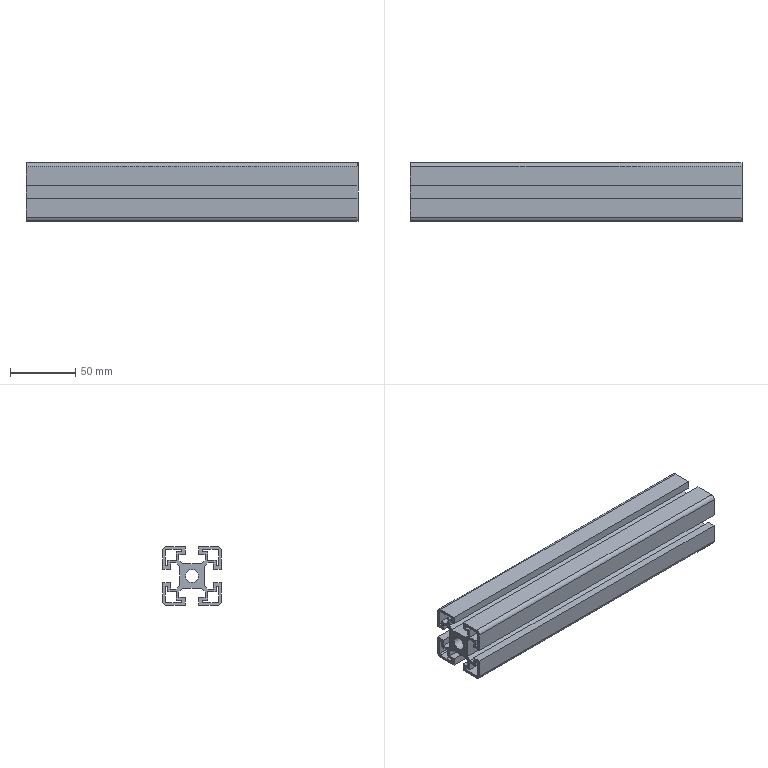Part | STEP file | bosch_3842990520_akhtc56kol25hyvavz80csddc | 1 solid | 87 faces | box 255 x 45 x 45 mm | volume 208524 mm3 | plane 78 | cylinder 9 | commonest cylinder face diameters 2 x4 6 x4 10 x1